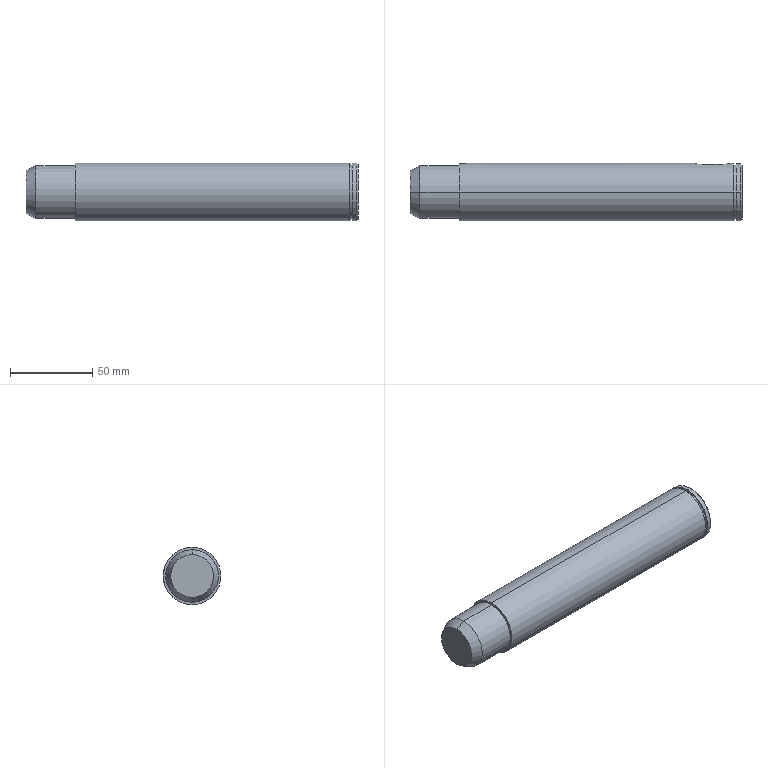Part | STEP file | 02-Support shaft 2 | 1 solid | 22 faces | box 201.5 x 35 x 35 mm | volume 187096 mm3 | cylinder 10 | plane 8 | cone 4 | commonest cylinder face diameters 35 x4 10 x2 32 x2 33 x2